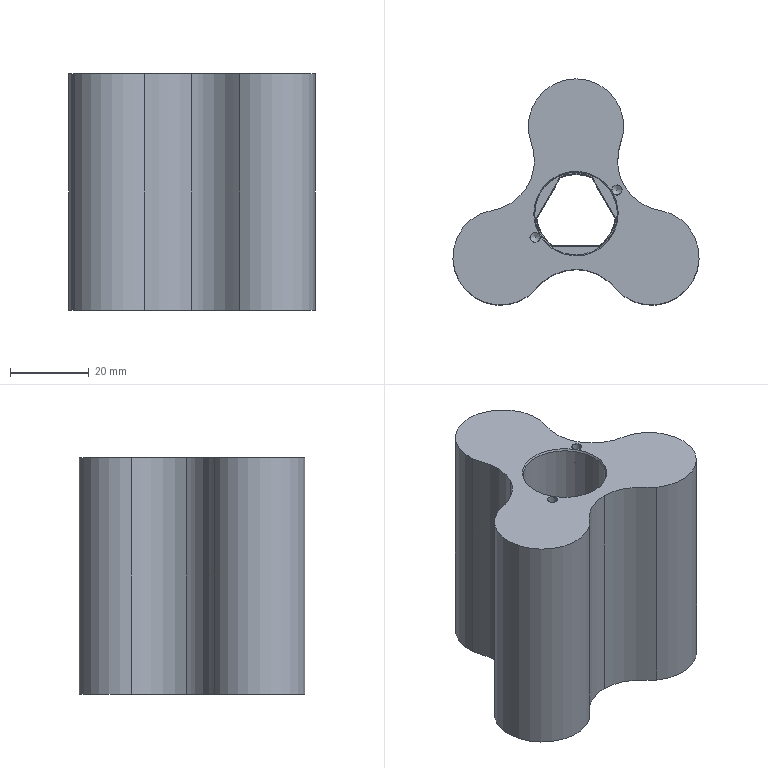NC program | NX | posted with a generic post | part box 62.563 x 57.43 x 60 mm
Lines 7568 to 8402 of 9902:
(CUTTER_COMP_12 , TOOL : D12)
N15128 T12 M6
N15130 G54
N15132 G17 G0 G90 X-1.396 Y-22.855 S5000 M3
N15134 G43 Z30. H12
N15136 Z1.
N15138 G94 G1 Z-1. F1250.
N15140 G41 X-1.489 Y-22.818 D12
N15142 X-4.167 Y-22.249
N15144 G3 X-5.308 Y-22.62 R1.2
N15146 G1 X-6.347 Y-23.775
N15148 G2 X-8.511 Y-25.728 R14.285
N15150 X-8.69 Y-25.859 R6.
N15152 X-26.736 Y5.406 R-18.126
N15154 X-23.436 Y6.459 R14.723
N15156 G3 X-21.483 Y6.922 R18.942
N15158 X-18.554 Y8.654 R7.232
N15160 X-16.551 Y13.607 R6.748
N15162 X-16.98 Y16.055 R8.604
N15164 G2 X-17.488 Y17.629 R75.664
N15166 X-18.049 Y20.45 R13.802
N15168 X18.05 Y20.455 R-18.126
N15170 X17.301 Y17.034 R14.72
N15172 G3 X16.839 Y15.566 R25.994
N15174 X16.603 Y12.628 R7.614
N15176 X19.715 Y7.735 R6.728
N15178 X21.889 Y6.804 R7.715
N15180 X23.436 Y6.459 R24.869
N15182 G2 X26.305 Y5.593 R14.617
N15184 G1 X26.317 Y5.58
N15186 G2 X26.74 Y5.404 R6.
N15188 X8.69 Y-25.86 R-18.126
N15190 G1 X8.532 Y-25.744
N15192 G2 X6.189 Y-23.599 R14.534
N15194 G3 X4.983 Y-22.293 R23.907
N15196 X2.441 Y-20.612 R7.51
N15198 X-3.528 Y-21.151 R6.743
N15200 X-5.308 Y-22.62 R8.35
N15202 X-5.568 Y-23.792 R1.2
N15204 G1 X-4.94 Y-25.785
N15206 G40
N15208 X-4.894 Y-25.873
N15210 Z1.
N15212 G0 X-1.396 Y-22.855 Z0.
N15214 G1 Z-2.
N15216 G41 X-1.489 Y-22.818
N15218 X-4.167 Y-22.249
N15220 G3 X-5.308 Y-22.62 R1.2
N15222 G1 X-6.347 Y-23.775
N15224 G2 X-8.511 Y-25.728 R14.308
N15226 X-8.69 Y-25.859 R6.
N15228 X-26.736 Y5.406 R-18.126
N15230 X-23.436 Y6.459 R14.722
N15232 G3 X-21.483 Y6.922 R18.943
N15234 X-18.554 Y8.655 R7.232
N15236 X-16.551 Y13.607 R6.747
N15238 X-16.98 Y16.055 R8.604
N15240 G2 X-17.488 Y17.63 R75.51
N15242 X-18.049 Y20.447 R13.797
N15244 X18.05 Y20.455 R-18.126
N15246 X17.301 Y17.034 R14.718
N15248 G3 X16.839 Y15.566 R25.986
N15250 X16.603 Y12.628 R7.614
N15252 X19.714 Y7.736 R6.728
N15254 X21.891 Y6.803 R7.714
N15256 X23.436 Y6.459 R24.945
N15258 G2 X26.305 Y5.593 R14.618
N15260 G1 X26.317 Y5.58
N15262 G2 X26.74 Y5.404 R6.
N15264 X8.69 Y-25.86 R-18.126
N15266 G1 X8.532 Y-25.744
N15268 G2 X6.189 Y-23.599 R14.532
N15270 G3 X4.983 Y-22.293 R23.906
N15272 X2.441 Y-20.612 R7.51
N15274 X-3.528 Y-21.151 R6.743
N15276 X-5.308 Y-22.62 R8.35
N15278 X-5.568 Y-23.792 R1.2
N15280 G1 X-4.94 Y-25.785
N15282 G40
N15284 X-4.894 Y-25.873
N15286 Z0.
N15288 G0 X-1.396 Y-22.855 Z-1.
N15290 G1 Z-3.
N15292 G41 X-1.489 Y-22.818
N15294 X-4.167 Y-22.249
N15296 G3 X-5.308 Y-22.62 R1.2
N15298 G1 X-6.347 Y-23.775
N15300 G2 X-8.511 Y-25.728 R14.304
N15302 X-8.69 Y-25.859 R6.
N15304 X-26.736 Y5.406 R-18.126
N15306 X-23.436 Y6.459 R14.721
N15308 G3 X-21.483 Y6.922 R18.944
N15310 X-18.554 Y8.655 R7.231
N15312 X-16.551 Y13.607 R6.747
N15314 X-16.98 Y16.055 R8.604
N15316 G2 X-17.488 Y17.631 R75.358
N15318 X-18.049 Y20.445 R13.792
N15320 X18.05 Y20.455 R-18.126
N15322 X17.301 Y17.034 R14.716
N15324 G3 X16.839 Y15.566 R25.977
N15326 X16.603 Y12.628 R7.614
N15328 X19.713 Y7.737 R6.728
N15330 X21.892 Y6.803 R7.714
N15332 X23.436 Y6.459 R25.021
N15334 G2 X26.305 Y5.593 R14.619
N15336 G1 X26.317 Y5.58
N15338 G2 X26.74 Y5.404 R6.
N15340 X8.69 Y-25.86 R-18.126
N15342 G1 X8.532 Y-25.744
N15344 G2 X6.189 Y-23.599 R14.531
N15346 G3 X4.983 Y-22.293 R23.905
N15348 X2.441 Y-20.612 R7.51
N15350 X-3.528 Y-21.151 R6.743
N15352 X-5.308 Y-22.62 R8.349
N15354 X-5.568 Y-23.792 R1.2
N15356 G1 X-4.94 Y-25.785
N15358 G40
N15360 X-4.894 Y-25.873
N15362 Z-1.
N15364 G0 X-1.589 Y-22.935 Z-2.
N15366 G1 Z-4.
N15368 G41 X-1.681 Y-22.895
N15370 X-4.153 Y-22.288
N15372 G3 X-5.305 Y-22.623 R1.2
N15374 X-6.189 Y-23.599 R23.026
N15376 G2 X-8.511 Y-25.728 R14.474
N15378 X-8.69 Y-25.859 R6.
N15380 X-26.736 Y5.406 R-18.126
N15382 X-23.436 Y6.459 R14.72
N15384 G3 X-21.483 Y6.922 R18.945
N15386 X-18.554 Y8.655 R7.231
N15388 X-16.551 Y13.607 R6.747
N15390 X-16.98 Y16.055 R8.604
N15392 G2 X-17.489 Y17.632 R75.206
N15394 X-18.049 Y20.443 R13.787
N15396 X18.05 Y20.455 R-18.126
N15398 X17.301 Y17.034 R14.714
N15400 G3 X16.839 Y15.566 R25.969
N15402 X16.603 Y12.628 R7.615
N15404 X19.712 Y7.737 R6.728
N15406 X21.893 Y6.802 R7.713
N15408 X23.436 Y6.459 R25.097
N15410 G2 X26.305 Y5.593 R14.621
N15412 G1 X26.317 Y5.58
N15414 G2 X26.74 Y5.404 R6.
N15416 X8.69 Y-25.86 R-18.126
N15418 G1 X8.532 Y-25.744
N15420 G2 X6.189 Y-23.599 R14.529
N15422 G3 X4.983 Y-22.293 R23.904
N15424 X2.441 Y-20.612 R7.51
N15426 X-2.93 Y-20.826 R6.728
N15428 X-4.883 Y-22.194 R7.566
N15430 X-5.305 Y-22.623 R23.026
N15432 X-5.591 Y-23.788 R1.2
N15434 G1 X-4.994 Y-25.841
N15436 G40
N15438 X-4.95 Y-25.931
N15440 Z-2.
N15442 G0 X-1.589 Y-22.935 Z-3.
N15444 G1 Z-5.
N15446 G41 X-1.681 Y-22.895
N15448 X-4.153 Y-22.288
N15450 G3 X-5.305 Y-22.623 R1.2
N15452 X-6.189 Y-23.599 R23.029
N15454 G2 X-8.511 Y-25.728 R14.473
N15456 X-8.69 Y-25.859 R6.
N15458 X-26.736 Y5.406 R-18.126
N15460 X-23.436 Y6.459 R14.719
N15462 G3 X-21.483 Y6.922 R18.946
N15464 X-18.554 Y8.655 R7.231
N15466 X-16.551 Y13.607 R6.747
N15468 X-16.98 Y16.055 R8.604
N15470 G2 X-17.489 Y17.633 R75.055
N15472 X-18.049 Y20.44 R13.782
N15474 X18.05 Y20.455 R-18.126
N15476 X17.301 Y17.034 R14.712
N15478 G3 X16.839 Y15.566 R25.961
N15480 X16.603 Y12.628 R7.615
N15482 X19.711 Y7.738 R6.728
N15484 X21.895 Y6.802 R7.713
N15486 X23.436 Y6.459 R25.175
N15488 G2 X26.305 Y5.593 R14.622
N15490 G1 X26.317 Y5.58
N15492 G2 X26.74 Y5.404 R6.
N15494 X8.69 Y-25.86 R-18.126
N15496 G1 X8.532 Y-25.744
N15498 G2 X6.189 Y-23.599 R14.528
N15500 G3 X4.983 Y-22.293 R23.903
N15502 X2.441 Y-20.612 R7.51
N15504 X-2.93 Y-20.826 R6.728
N15506 X-4.883 Y-22.194 R7.566
N15508 X-5.305 Y-22.623 R23.029
N15510 X-5.591 Y-23.788 R1.2
N15512 G1 X-4.994 Y-25.841
N15514 G40
N15516 X-4.95 Y-25.931
N15518 Z-3.
N15520 G0 X-1.589 Y-22.935 Z-4.
N15522 G1 Z-6.
N15524 G41 X-1.681 Y-22.895
N15526 X-4.153 Y-22.288
N15528 G3 X-5.305 Y-22.623 R1.2
N15530 X-6.189 Y-23.599 R23.031
N15532 G2 X-8.511 Y-25.728 R14.471
N15534 X-8.69 Y-25.859 R6.
N15536 X-26.736 Y5.406 R-18.126
N15538 X-23.436 Y6.459 R14.719
N15540 G3 X-21.483 Y6.922 R18.947
N15542 X-18.554 Y8.655 R7.228
N15544 X-16.551 Y13.607 R6.747
N15546 X-16.98 Y16.055 R8.604
N15548 G2 X-17.488 Y17.63 R74.904
N15550 X-18.05 Y20.455 R13.816
N15552 X18.05 Y20.455 R-18.126
N15554 X17.301 Y17.034 R14.711
N15556 G3 X16.839 Y15.566 R25.952
N15558 X16.603 Y12.628 R7.615
N15560 X19.71 Y7.738 R6.728
N15562 X21.896 Y6.802 R7.712
N15564 X23.436 Y6.459 R25.252
N15566 G2 X26.305 Y5.593 R14.623
N15568 G1 X26.317 Y5.58
N15570 G2 X26.74 Y5.404 R6.
N15572 X8.69 Y-25.86 R-18.126
N15574 G1 X8.532 Y-25.744
N15576 G2 X6.189 Y-23.599 R14.526
N15578 G3 X4.983 Y-22.293 R23.902
N15580 X2.441 Y-20.612 R7.51
N15582 X-2.93 Y-20.826 R6.728
N15584 X-4.883 Y-22.194 R7.566
N15586 X-5.305 Y-22.623 R23.031
N15588 X-5.591 Y-23.788 R1.2
N15590 G1 X-4.994 Y-25.841
N15592 G40
N15594 X-4.95 Y-25.931
N15596 Z-4.
N15598 G0 X-1.589 Y-22.935 Z-5.
N15600 G1 Z-7.
N15602 G41 X-1.681 Y-22.895
N15604 X-4.153 Y-22.288
N15606 G3 X-5.305 Y-22.623 R1.2
N15608 X-6.189 Y-23.599 R23.034
N15610 G2 X-8.511 Y-25.728 R14.47
N15612 X-8.69 Y-25.859 R6.
N15614 X-26.736 Y5.406 R-18.126
N15616 X-23.436 Y6.459 R14.718
N15618 G3 X-21.483 Y6.922 R18.834
N15620 X-18.554 Y8.655 R7.228
N15622 X-16.551 Y13.607 R6.747
N15624 X-16.98 Y16.055 R8.604
N15626 G2 X-17.488 Y17.631 R74.754
N15628 X-18.05 Y20.452 R13.811
N15630 X18.05 Y20.455 R-18.126
N15632 X17.301 Y17.034 R14.709
N15634 G3 X16.839 Y15.566 R25.944
N15636 X16.603 Y12.628 R7.616
N15638 X19.719 Y7.733 R6.728
N15640 X22.088 Y6.753 R7.894
N15642 X23.436 Y6.459 R25.33
N15644 G2 X26.305 Y5.593 R14.624
N15646 G1 X26.317 Y5.58
N15648 G2 X26.74 Y5.404 R6.
N15650 X8.69 Y-25.86 R-18.126
N15652 G1 X8.532 Y-25.744
N15654 G2 X6.189 Y-23.599 R14.525
N15656 G3 X4.983 Y-22.293 R23.901
N15658 X2.441 Y-20.612 R7.509
N15660 X-2.93 Y-20.826 R6.728
N15662 X-4.883 Y-22.194 R7.566
N15664 X-5.305 Y-22.623 R23.034
N15666 X-5.591 Y-23.788 R1.2
N15668 G1 X-4.994 Y-25.841
N15670 G40
N15672 X-4.95 Y-25.931
N15674 Z-5.
N15676 G0 X-1.589 Y-22.935 Z-6.
N15678 G1 Z-8.
N15680 G41 X-1.681 Y-22.895
N15682 X-4.153 Y-22.288
N15684 G3 X-5.305 Y-22.623 R1.2
N15686 X-6.189 Y-23.599 R23.036
N15688 G2 X-8.511 Y-25.728 R14.469
N15690 X-8.69 Y-25.859 R6.
N15692 X-26.736 Y5.406 R-18.126
N15694 X-23.436 Y6.459 R14.692
N15696 G3 X-21.483 Y6.922 R18.832
N15698 X-18.554 Y8.655 R7.228
N15700 X-16.551 Y13.607 R6.747
N15702 X-16.98 Y16.055 R8.604
N15704 G2 X-17.489 Y17.632 R74.605
N15706 X-18.049 Y20.45 R13.806
N15708 X18.05 Y20.455 R-18.126
N15710 X17.301 Y17.034 R14.707
N15712 G3 X16.839 Y15.566 R25.936
N15714 X16.603 Y12.628 R7.616
N15716 X19.72 Y7.733 R6.728
N15718 X22.088 Y6.753 R7.897
N15720 X23.436 Y6.459 R25.409
N15722 G2 X26.305 Y5.593 R14.626
N15724 G1 X26.317 Y5.58
N15726 G2 X26.74 Y5.404 R6.
N15728 X8.69 Y-25.86 R-18.126
N15730 G1 X8.532 Y-25.744
N15732 G2 X6.189 Y-23.599 R14.523
N15734 G3 X4.983 Y-22.293 R23.9
N15736 X2.441 Y-20.612 R7.509
N15738 X-2.93 Y-20.827 R6.727
N15740 X-4.883 Y-22.194 R7.566
N15742 X-5.305 Y-22.623 R23.036
N15744 X-5.591 Y-23.788 R1.2
N15746 G1 X-4.994 Y-25.841
N15748 G40
N15750 X-4.95 Y-25.931
N15752 Z-6.
N15754 G0 X-1.589 Y-22.935 Z-7.
N15756 G1 Z-9.
N15758 G41 X-1.681 Y-22.895
N15760 X-4.153 Y-22.288
N15762 G3 X-5.305 Y-22.623 R1.2
N15764 X-6.189 Y-23.599 R23.039
N15766 G2 X-8.511 Y-25.728 R14.468
N15768 X-8.69 Y-25.859 R6.
N15770 X-26.736 Y5.406 R-18.126
N15772 X-23.436 Y6.459 R14.691
N15774 G3 X-21.483 Y6.922 R18.831
N15776 X-18.554 Y8.655 R7.227
N15778 X-16.551 Y13.607 R6.747
N15780 X-16.981 Y16.055 R8.604
N15782 G2 X-17.489 Y17.633 R74.456
N15784 X-18.049 Y20.447 R13.801
N15786 X18.05 Y20.455 R-18.126
N15788 X17.301 Y17.034 R14.705
N15790 G3 X16.839 Y15.566 R25.927
N15792 X16.603 Y12.628 R7.616
N15794 X19.72 Y7.733 R6.728
N15796 X22.088 Y6.753 R7.899
N15798 X23.436 Y6.459 R25.488
N15800 G2 X26.305 Y5.593 R14.627
N15802 G1 X26.317 Y5.58
N15804 G2 X26.74 Y5.404 R6.
N15806 X8.69 Y-25.86 R-18.126
N15808 G1 X8.532 Y-25.744
N15810 G2 X6.189 Y-23.599 R14.522
N15812 G3 X4.983 Y-22.293 R23.899
N15814 X2.441 Y-20.612 R7.509
N15816 X-2.93 Y-20.827 R6.727
N15818 X-4.883 Y-22.194 R7.566
N15820 X-5.305 Y-22.623 R23.039
N15822 X-5.591 Y-23.788 R1.2
N15824 G1 X-4.994 Y-25.841
N15826 G40
N15828 X-4.95 Y-25.931
N15830 Z-7.
N15832 G0 X-1.589 Y-22.935 Z-8.
N15834 G1 Z-10.
N15836 G41 X-1.681 Y-22.895
N15838 X-4.153 Y-22.288
N15840 G3 X-5.305 Y-22.623 R1.2
N15842 X-6.189 Y-23.599 R23.041
N15844 G2 X-8.511 Y-25.728 R14.466
N15846 X-8.69 Y-25.859 R6.
N15848 X-26.736 Y5.406 R-18.126
N15850 X-23.436 Y6.46 R14.69
N15852 G3 X-21.483 Y6.922 R18.829
N15854 X-18.554 Y8.655 R7.227
N15856 X-16.551 Y13.607 R6.746
N15858 X-16.981 Y16.055 R8.604
N15860 G2 X-17.489 Y17.634 R74.308
N15862 X-18.049 Y20.445 R13.796
N15864 X18.05 Y20.455 R-18.126
N15866 X17.301 Y17.034 R14.703
N15868 G3 X16.84 Y15.566 R25.919
N15870 X16.603 Y12.628 R7.617
N15872 X19.72 Y7.733 R6.728
N15874 X22.088 Y6.753 R7.902
N15876 X23.436 Y6.459 R25.567
N15878 G2 X26.305 Y5.593 R14.628
N15880 G1 X26.317 Y5.58
N15882 G2 X26.74 Y5.404 R6.
N15884 X8.69 Y-25.86 R-18.126
N15886 G1 X8.532 Y-25.744
N15888 G2 X6.189 Y-23.599 R14.52
N15890 G3 X4.983 Y-22.293 R23.898
N15892 X2.441 Y-20.612 R7.509
N15894 X-2.93 Y-20.827 R6.727
N15896 X-4.883 Y-22.194 R7.566
N15898 X-5.305 Y-22.623 R23.041
N15900 X-5.591 Y-23.788 R1.2
N15902 G1 X-4.994 Y-25.841
N15904 G40
N15906 X-4.95 Y-25.931
N15908 Z-8.
N15910 G0 X-1.589 Y-22.935 Z-9.
N15912 G1 Z-11.
N15914 G41 X-1.681 Y-22.895
N15916 X-4.152 Y-22.288
N15918 G3 X-5.305 Y-22.623 R1.2
N15920 X-6.189 Y-23.599 R23.044
N15922 G2 X-8.511 Y-25.728 R14.465
N15924 X-8.69 Y-25.859 R6.
N15926 X-26.736 Y5.406 R-18.126
N15928 X-23.436 Y6.46 R14.689
N15930 G3 X-21.483 Y6.922 R18.828
N15932 X-18.554 Y8.655 R7.227
N15934 X-16.551 Y13.607 R6.746
N15936 X-16.981 Y16.055 R8.604
N15938 G2 X-17.49 Y17.635 R74.005
N15940 X-18.049 Y20.442 R13.791
N15942 X18.05 Y20.455 R-18.126
N15944 X17.301 Y17.034 R14.701
N15946 G3 X16.84 Y15.566 R25.911
N15948 X16.603 Y12.628 R7.616
N15950 X19.72 Y7.733 R6.728
N15952 X22.088 Y6.753 R7.904
N15954 X23.436 Y6.459 R25.647
N15956 G2 X26.305 Y5.593 R14.63
N15958 G1 X26.317 Y5.58
N15960 G2 X26.74 Y5.404 R6.
N15962 X8.69 Y-25.86 R-18.126
N15964 G1 X8.532 Y-25.744
N15966 G2 X6.189 Y-23.599 R14.519
N15968 G3 X4.983 Y-22.293 R23.897
N15970 X2.441 Y-20.612 R7.509
N15972 X-2.93 Y-20.827 R6.724
N15974 X-4.883 Y-22.194 R7.566
N15976 X-5.305 Y-22.623 R23.044
N15978 X-5.591 Y-23.788 R1.2
N15980 G1 X-4.994 Y-25.841
N15982 G40
N15984 X-4.95 Y-25.931
N15986 Z-9.
N15988 G0 X-1.589 Y-22.935 Z-10.
N15990 G1 Z-12.
N15992 G41 X-1.681 Y-22.895
N15994 X-4.152 Y-22.288
N15996 G3 X-5.305 Y-22.623 R1.2
N15998 X-6.189 Y-23.599 R23.046
N16000 G2 X-8.511 Y-25.728 R14.464
N16002 X-8.69 Y-25.859 R6.
N16004 X-26.736 Y5.406 R-18.126
N16006 X-23.436 Y6.46 R14.689
N16008 G3 X-21.483 Y6.922 R18.826
N16010 X-18.554 Y8.655 R7.227
N16012 X-16.551 Y13.607 R6.746
N16014 X-16.981 Y16.055 R8.604
N16016 G2 X-17.49 Y17.636 R73.885
N16018 X-18.048 Y20.44 R13.786
N16020 X18.05 Y20.455 R-18.126
N16022 X17.301 Y17.034 R14.699
N16024 G3 X16.84 Y15.566 R25.903
N16026 X16.603 Y12.628 R7.616
N16028 X19.72 Y7.733 R6.728
N16030 X22.088 Y6.753 R7.907
N16032 X23.436 Y6.46 R25.728
N16034 G2 X26.305 Y5.593 R14.631
N16036 G1 X26.317 Y5.58
N16038 G2 X26.74 Y5.404 R6.
N16040 X8.69 Y-25.86 R-18.126
N16042 G1 X8.532 Y-25.744
N16044 G2 X6.189 Y-23.599 R14.517
N16046 G3 X4.983 Y-22.293 R23.896
N16048 X2.441 Y-20.612 R7.509
N16050 X-2.93 Y-20.827 R6.727
N16052 X-4.883 Y-22.194 R7.566
N16054 X-5.305 Y-22.623 R23.046
N16056 X-5.591 Y-23.788 R1.2
N16058 G1 X-4.994 Y-25.841
N16060 G40
N16062 X-4.95 Y-25.931
N16064 Z-10.
N16066 G0 X-1.589 Y-22.935 Z-11.
N16068 G1 Z-13.
N16070 G41 X-1.68 Y-22.895
N16072 X-4.152 Y-22.288
N16074 G3 X-5.305 Y-22.623 R1.2
N16076 X-6.189 Y-23.599 R23.049
N16078 G2 X-8.511 Y-25.728 R14.463
N16080 X-8.69 Y-25.859 R6.
N16082 X-26.736 Y5.406 R-18.126
N16084 X-23.436 Y6.46 R14.688
N16086 G3 X-21.483 Y6.922 R18.825
N16088 X-18.554 Y8.655 R7.226
N16090 X-16.551 Y13.607 R6.746
N16092 X-16.981 Y16.055 R8.604
N16094 G2 X-17.49 Y17.637 R73.765
N16096 X-18.048 Y20.437 R13.78
N16098 X18.05 Y20.455 R-18.126
N16100 X17.301 Y17.034 R14.698
N16102 G3 X16.84 Y15.566 R25.894
N16104 X16.603 Y12.628 R7.615
N16106 X19.72 Y7.733 R6.728
N16108 X22.088 Y6.753 R7.909
N16110 X23.436 Y6.46 R25.809
N16112 G2 X26.305 Y5.593 R14.632
N16114 G1 X26.317 Y5.58
N16116 G2 X26.74 Y5.404 R6.
N16118 X8.69 Y-25.86 R-18.126
N16120 G1 X8.532 Y-25.744
N16122 G2 X6.189 Y-23.599 R14.516
N16124 G3 X4.983 Y-22.293 R23.895
N16126 X2.441 Y-20.612 R7.509
N16128 X-2.93 Y-20.827 R6.727
N16130 X-4.883 Y-22.194 R7.566
N16132 X-5.305 Y-22.623 R23.049
N16134 X-5.591 Y-23.788 R1.2
N16136 G1 X-4.994 Y-25.841
N16138 G40
N16140 X-4.95 Y-25.931
N16142 Z-11.
N16144 G0 X-1.589 Y-22.935 Z-12.
N16146 G1 Z-14.
N16148 G41 X-1.68 Y-22.895
N16150 X-4.152 Y-22.288
N16152 G3 X-5.305 Y-22.623 R1.2
N16154 X-6.188 Y-23.599 R23.051
N16156 G2 X-8.511 Y-25.728 R14.461
N16158 X-8.69 Y-25.859 R6.
N16160 X-26.736 Y5.406 R-18.126
N16162 X-23.436 Y6.46 R14.687
N16164 G3 X-21.483 Y6.922 R18.823
N16166 X-18.554 Y8.655 R7.226
N16168 X-16.551 Y13.607 R6.746
N16170 X-16.981 Y16.055 R8.604
N16172 G2 X-17.491 Y17.638 R73.645
N16174 X-18.048 Y20.435 R13.775
N16176 X18.05 Y20.455 R-18.126
N16178 X17.302 Y17.034 R14.696
N16180 G3 X16.84 Y15.566 R25.886
N16182 X16.603 Y12.628 R7.615
N16184 X19.72 Y7.733 R6.729
N16186 X22.088 Y6.753 R7.912
N16188 X23.436 Y6.46 R25.89
N16190 G2 X26.305 Y5.593 R14.634
N16192 G1 X26.317 Y5.58
N16194 G2 X26.74 Y5.404 R6.
N16196 X8.69 Y-25.86 R-18.126
N16198 G1 X8.532 Y-25.744
N16200 G2 X6.189 Y-23.599 R14.514
N16202 G3 X4.983 Y-22.293 R23.894
N16204 X2.441 Y-20.612 R7.508
N16206 X-2.93 Y-20.827 R6.727
N16208 X-4.883 Y-22.194 R7.566
N16210 X-5.305 Y-22.623 R23.051
N16212 X-5.591 Y-23.788 R1.2
N16214 G1 X-4.994 Y-25.841
N16216 G40
N16218 X-4.95 Y-25.931
N16220 Z-12.
N16222 G0 X-1.589 Y-22.935 Z-13.
N16224 G1 Z-15.
N16226 G41 X-1.68 Y-22.895
N16228 X-4.152 Y-22.288
N16230 G3 X-5.305 Y-22.623 R1.2
N16232 X-6.188 Y-23.599 R23.054
N16234 G2 X-8.511 Y-25.728 R14.46
N16236 X-8.69 Y-25.859 R6.
N16238 X-26.736 Y5.406 R-18.126
N16240 X-23.436 Y6.46 R14.686
N16242 G3 X-21.483 Y6.922 R18.822
N16244 X-18.554 Y8.655 R7.226
N16246 X-16.552 Y13.607 R6.746
N16248 X-16.981 Y16.055 R8.604
N16250 G2 X-17.491 Y17.639 R73.525
N16252 X-18.048 Y20.433 R13.77
N16254 X18.05 Y20.455 R-18.126
N16256 X17.302 Y17.034 R14.694
N16258 G3 X16.84 Y15.566 R25.878
N16260 X16.603 Y12.628 R7.622
N16262 X19.72 Y7.733 R6.729
N16264 X22.088 Y6.753 R7.914
N16266 X23.436 Y6.46 R25.973
N16268 G2 X26.305 Y5.593 R14.635
N16270 G1 X26.317 Y5.58
N16272 G2 X26.74 Y5.404 R6.
N16274 X8.69 Y-25.86 R-18.126
N16276 G1 X8.532 Y-25.744
N16278 G2 X6.189 Y-23.599 R14.513
N16280 G3 X4.983 Y-22.293 R23.893
N16282 X2.441 Y-20.613 R7.508
N16284 X-2.93 Y-20.827 R6.726
N16286 X-4.883 Y-22.194 R7.566
N16288 X-5.305 Y-22.623 R23.054
N16290 X-5.591 Y-23.788 R1.2
N16292 G1 X-4.994 Y-25.841
N16294 G40
N16296 X-4.95 Y-25.931
N16298 Z-13.
N16300 G0 X-1.589 Y-22.935 Z-14.
N16302 G1 Z-16.
N16304 G41 X-1.68 Y-22.895
N16306 X-4.152 Y-22.288
N16308 G3 X-5.305 Y-22.623 R1.2
N16310 X-6.188 Y-23.599 R23.056
N16312 G2 X-8.511 Y-25.728 R14.459
N16314 X-8.69 Y-25.859 R6.
N16316 X-26.736 Y5.406 R-18.126
N16318 X-23.436 Y6.46 R14.685
N16320 G3 X-21.483 Y6.922 R18.821
N16322 X-18.554 Y8.655 R7.226
N16324 X-16.552 Y13.607 R6.746
N16326 X-16.981 Y16.055 R8.604
N16328 G2 X-17.491 Y17.64 R73.406
N16330 X-18.048 Y20.43 R13.764
N16332 X18.05 Y20.455 R-18.126
N16334 X17.302 Y17.034 R14.692
N16336 G3 X16.84 Y15.566 R25.869
N16338 X16.603 Y12.628 R7.622
N16340 X19.72 Y7.733 R6.729
N16342 X22.088 Y6.753 R7.907
N16344 X23.436 Y6.46 R26.055
N16346 G2 X26.305 Y5.593 R14.636
N16348 G1 X26.317 Y5.58
N16350 G2 X26.74 Y5.404 R6.
N16352 X8.69 Y-25.86 R-18.126
N16354 G1 X8.532 Y-25.744
N16356 G2 X6.189 Y-23.599 R14.511
N16358 G3 X4.983 Y-22.293 R23.892
N16360 X2.441 Y-20.613 R7.508
N16362 X-2.93 Y-20.827 R6.726
N16364 X-4.883 Y-22.194 R7.566
N16366 X-5.305 Y-22.623 R23.056
N16368 X-5.591 Y-23.788 R1.2
N16370 G1 X-4.994 Y-25.841
N16372 G40
N16374 X-4.95 Y-25.931
N16376 Z-14.
N16378 G0 X-1.589 Y-22.935 Z-15.
N16380 G1 Z-17.
N16382 G41 X-1.68 Y-22.895
N16384 X-4.152 Y-22.288
N16386 G3 X-5.305 Y-22.623 R1.2
N16388 X-6.188 Y-23.599 R23.059
N16390 G2 X-8.511 Y-25.728 R14.458
N16392 X-8.69 Y-25.859 R6.
N16394 X-26.736 Y5.406 R-18.126
N16396 X-23.436 Y6.46 R14.684
N16398 G3 X-21.483 Y6.923 R18.819
N16400 X-18.554 Y8.655 R7.225
N16402 X-16.552 Y13.607 R6.746
N16404 X-16.981 Y16.055 R8.604
N16406 G2 X-17.492 Y17.641 R73.288
N16408 X-18.047 Y20.428 R13.759
N16410 X18.05 Y20.455 R-18.126
N16412 X17.302 Y17.034 R14.69
N16414 G3 X16.84 Y15.566 R25.861
N16416 X16.603 Y12.628 R7.621
N16418 X20.507 Y7.303 R6.763
N16420 X22.46 Y6.663 R9.349
N16422 G2 X24.056 Y6.321 R59.754
N16424 X26.305 Y5.594 R13.414
N16426 G1 X26.317 Y5.58
N16428 G2 X26.74 Y5.404 R6.
N16430 X8.69 Y-25.86 R-18.126
N16432 G1 X8.532 Y-25.744
N16434 G2 X6.189 Y-23.599 R14.509
N16436 G3 X4.983 Y-22.292 R23.891
N16438 X2.441 Y-20.613 R7.508
N16440 X-2.93 Y-20.827 R6.726
N16442 X-4.883 Y-22.194 R7.566
N16444 X-5.305 Y-22.623 R23.059
N16446 X-5.591 Y-23.788 R1.2
N16448 G1 X-4.994 Y-25.841
N16450 G40
N16452 X-4.95 Y-25.931
N16454 Z-15.
N16456 G0 X-1.589 Y-22.935 Z-16.
N16458 G1 Z-18.
N16460 G41 X-1.68 Y-22.895
N16462 X-4.152 Y-22.288
N16464 G3 X-5.305 Y-22.623 R1.2
N16466 X-6.188 Y-23.599 R23.062
N16468 G2 X-8.511 Y-25.728 R14.456
N16470 X-8.69 Y-25.859 R6.
N16472 X-26.736 Y5.406 R-18.126
N16474 X-23.436 Y6.46 R14.683
N16476 G3 X-21.483 Y6.923 R18.818
N16478 X-18.554 Y8.655 R7.225
N16480 X-16.552 Y13.607 R6.746
N16482 X-16.981 Y16.055 R8.604
N16484 G2 X-17.492 Y17.642 R73.169
N16486 X-18.047 Y20.425 R13.754
N16488 X18.05 Y20.455 R-18.126
N16490 X17.302 Y17.034 R14.688
N16492 G3 X16.84 Y15.566 R25.853
N16494 X16.603 Y12.628 R7.621
N16496 X20.507 Y7.303 R6.763
N16498 X22.46 Y6.663 R9.348
N16500 G2 X24.057 Y6.321 R59.655
N16502 X26.305 Y5.594 R13.413
N16504 G1 X26.317 Y5.58
N16506 G2 X26.74 Y5.404 R6.
N16508 X8.69 Y-25.86 R-18.126
N16510 G1 X8.532 Y-25.744
N16512 G2 X6.189 Y-23.599 R14.508
N16514 G3 X4.983 Y-22.292 R23.89
N16516 X2.441 Y-20.613 R7.508
N16518 X-2.93 Y-20.827 R6.726
N16520 X-4.883 Y-22.194 R7.567
N16522 X-5.305 Y-22.623 R23.062
N16524 X-5.591 Y-23.789 R1.2
N16526 G1 X-4.994 Y-25.841
N16528 G40
N16530 X-4.95 Y-25.931
N16532 Z-16.
N16534 G0 X-1.589 Y-22.935 Z-17.
N16536 G1 Z-19.
N16538 G41 X-1.68 Y-22.895
N16540 X-4.152 Y-22.288
N16542 G3 X-5.305 Y-22.623 R1.2
N16544 X-6.188 Y-23.599 R23.064
N16546 G2 X-8.511 Y-25.728 R14.455
N16548 X-8.69 Y-25.859 R6.
N16550 X-26.736 Y5.406 R-18.126
N16552 X-23.436 Y6.46 R14.682
N16554 G3 X-21.483 Y6.923 R18.816
N16556 X-18.554 Y8.655 R7.225
N16558 X-16.552 Y13.607 R6.745
N16560 X-16.981 Y16.055 R8.604
N16562 G2 X-17.492 Y17.643 R73.051
N16564 X-18.047 Y20.423 R13.749
N16566 X18.05 Y20.455 R-18.126
N16568 X17.302 Y17.034 R14.686
N16570 G3 X16.84 Y15.566 R25.845
N16572 X16.603 Y12.628 R7.62
N16574 X20.507 Y7.303 R6.763
N16576 X22.46 Y6.663 R9.347
N16578 G2 X24.058 Y6.32 R59.555
N16580 X26.305 Y5.594 R13.412
N16582 G1 X26.317 Y5.58
N16584 G2 X26.74 Y5.404 R6.
N16586 X8.69 Y-25.86 R-18.126
N16588 G1 X8.532 Y-25.744
N16590 G2 X6.189 Y-23.599 R14.506
N16592 G3 X4.983 Y-22.292 R23.889
N16594 X2.441 Y-20.613 R7.508
N16596 X-2.93 Y-20.827 R6.726
N16598 X-4.883 Y-22.194 R7.567
N16600 X-5.305 Y-22.623 R23.064
N16602 X-5.591 Y-23.789 R1.2
N16604 G1 X-4.994 Y-25.841
N16606 G40
N16608 X-4.95 Y-25.931
N16610 Z-17.
N16612 G0 X-1.589 Y-22.935 Z-18.
N16614 G1 Z-20.
N16616 G41 X-1.68 Y-22.895
N16618 X-4.152 Y-22.288
N16620 G3 X-5.305 Y-22.623 R1.2
N16622 X-6.188 Y-23.599 R23.067
N16624 G2 X-8.511 Y-25.728 R14.454
N16626 X-8.69 Y-25.859 R6.
N16628 X-26.736 Y5.406 R-18.126
N16630 X-23.436 Y6.46 R14.681
N16632 G3 X-21.483 Y6.923 R18.815
N16634 X-18.554 Y8.655 R7.225
N16636 X-16.552 Y13.607 R6.745
N16638 X-16.981 Y16.055 R8.604
N16640 G2 X-17.49 Y17.635 R72.934
N16642 X-18.05 Y20.453 R13.818
N16644 X18.05 Y20.455 R-18.126
N16646 X17.302 Y17.034 R14.685
N16648 G3 X16.84 Y15.566 R25.836
N16650 X16.603 Y12.628 R7.62
N16652 X20.507 Y7.303 R6.762
N16654 X22.46 Y6.663 R9.346
N16656 G2 X24.059 Y6.32 R59.456
N16658 X26.305 Y5.594 R13.411
N16660 G1 X26.317 Y5.58
N16662 G2 X26.74 Y5.404 R6.
N16664 X8.69 Y-25.86 R-18.126
N16666 G1 X8.532 Y-25.744
N16668 G2 X6.189 Y-23.599 R14.505
N16670 G3 X4.983 Y-22.292 R23.889
N16672 X2.441 Y-20.613 R7.508
N16674 X-2.93 Y-20.827 R6.726
N16676 X-4.883 Y-22.194 R7.567
N16678 X-5.305 Y-22.623 R23.067
N16680 X-5.591 Y-23.789 R1.2
N16682 G1 X-4.994 Y-25.841
N16684 G40
N16686 X-4.95 Y-25.931
N16688 Z-18.
N16690 G0 X-1.589 Y-22.935 Z-19.
N16692 G1 Z-21.
N16694 G41 X-1.68 Y-22.895
N16696 X-4.152 Y-22.288
N16698 G3 X-5.305 Y-22.623 R1.2
N16700 X-6.188 Y-23.599 R23.069
N16702 G2 X-8.511 Y-25.728 R14.453
N16704 X-8.69 Y-25.859 R6.
N16706 X-26.736 Y5.406 R-18.126
N16708 X-23.436 Y6.46 R14.68
N16710 G3 X-21.483 Y6.923 R18.813
N16712 X-18.554 Y8.655 R7.225
N16714 X-16.552 Y13.607 R6.745
N16716 X-16.981 Y16.055 R8.604
N16718 G2 X-17.49 Y17.636 R72.817
N16720 X-18.049 Y20.45 R13.813
N16722 X18.05 Y20.455 R-18.126
N16724 X17.302 Y17.034 R14.683
N16726 G3 X16.84 Y15.566 R25.828
N16728 X16.603 Y12.628 R7.619
N16730 X20.507 Y7.303 R6.765
N16732 X22.46 Y6.663 R9.344
N16734 G2 X24.06 Y6.32 R59.358
N16736 X26.305 Y5.594 R13.41
N16738 G1 X26.317 Y5.58
N16740 G2 X26.74 Y5.404 R6.
N16742 X8.69 Y-25.86 R-18.126
N16744 G1 X8.532 Y-25.744
N16746 G2 X6.189 Y-23.599 R14.503
N16748 G3 X4.983 Y-22.292 R23.888
N16750 X2.441 Y-20.613 R7.507
N16752 X-2.93 Y-20.827 R6.726
N16754 X-4.883 Y-22.194 R7.567
N16756 X-5.305 Y-22.623 R23.069
N16758 X-5.591 Y-23.789 R1.2
N16760 G1 X-4.994 Y-25.841
N16762 G40
N16764 X-4.95 Y-25.931
N16766 Z-19.
N16768 G0 X-1.588 Y-22.935 Z-20.
N16770 G1 Z-22.
N16772 G41 X-1.68 Y-22.895
N16774 X-4.152 Y-22.288
N16776 G3 X-5.305 Y-22.623 R1.2
N16778 X-6.188 Y-23.599 R23.072
N16780 G2 X-8.511 Y-25.728 R14.452
N16782 X-8.69 Y-25.859 R6.
N16784 X-26.736 Y5.406 R-18.126
N16786 X-23.436 Y6.46 R14.68
N16788 G3 X-21.483 Y6.923 R18.812
N16790 X-18.554 Y8.655 R7.224